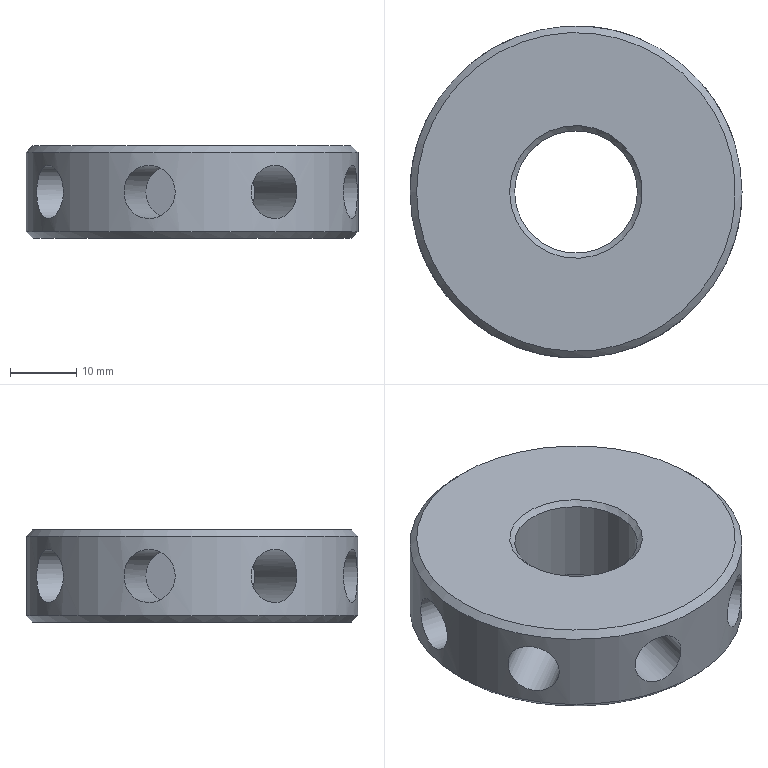Part | STEP file | 冲床-300配套压波_id1102_x_t | 1 solid | 24 faces | box 50 x 50 x 14 mm | volume 18346 mm3 | cylinder 10 | plane 10 | cone 4 | commonest cylinder face diameters 8 x8 18.5 x1 50 x1
STEP:
#1=CARTESIAN_POINT('',(1259.25,-86.,224.1));
#2=VERTEX_POINT('',#1);
#3=CARTESIAN_POINT('',(1250.,-86.,224.1));
#4=DIRECTION('',(0.,0.,-1.));
#5=DIRECTION('',(1.,0.,0.));
#6=AXIS2_PLACEMENT_3D('',#3,#4,#5);
#7=CIRCLE('',#6,9.25);
#8=EDGE_CURVE('',#2,#2,#7,.T.);
#9=ORIENTED_EDGE('',*,*,#8,.T.);
#10=EDGE_LOOP('',(#9));
#11=FACE_BOUND('',#10,.T.);
#12=CARTESIAN_POINT('',(1240.75,-86.,236.6));
#13=VERTEX_POINT('',#12);
#14=CARTESIAN_POINT('',(1250.,-86.,236.6));
#15=DIRECTION('',(0.,0.,1.));
#16=DIRECTION('',(-1.,0.,0.));
#17=AXIS2_PLACEMENT_3D('',#14,#15,#16);
#18=CIRCLE('',#17,9.25);
#19=EDGE_CURVE('',#13,#13,#18,.T.);
#20=ORIENTED_EDGE('',*,*,#19,.T.);
#21=EDGE_LOOP('',(#20));
#22=FACE_BOUND('',#21,.T.);
#23=CARTESIAN_POINT('',(1250.,-86.,224.35));
#24=DIRECTION('',(0.,0.,1.));
#25=DIRECTION('',(-1.,0.,0.));
#26=AXIS2_PLACEMENT_3D('',#23,#24,#25);
#27=CYLINDRICAL_SURFACE('',#26,9.25);
#28=ADVANCED_FACE('',(#11,#22),#27,.F.);
#29=CARTESIAN_POINT('',(1239.444,-79.03,230.35));
#30=VERTEX_POINT('',#29);
#31=CARTESIAN_POINT('',(1238.409,-82.894,230.35));
#32=DIRECTION('',(0.9659,-0.2588,0.));
#33=DIRECTION('',(0.2588,0.9659,0.));
#34=AXIS2_PLACEMENT_3D('',#31,#32,#33);
#35=CIRCLE('',#34,4.);
#36=EDGE_CURVE('',#30,#30,#35,.T.);
#37=ORIENTED_EDGE('',*,*,#36,.F.);
#38=EDGE_LOOP('',(#37));
#39=FACE_OUTER_BOUND('',#38,.T.);
#40=CARTESIAN_POINT('',(1238.409,-82.894,230.35));
#41=DIRECTION('',(0.9659,-0.2588,0.));
#42=DIRECTION('',(0.,0.,-1.));
#43=AXIS2_PLACEMENT_3D('',#40,#41,#42);
#44=PLANE('',#43);
#45=ADVANCED_FACE('',(#39),#44,.F.);
#46=CARTESIAN_POINT('',(1225.665,-80.271,234.276));
#47=VERTEX_POINT('',#46);
#48=CARTESIAN_POINT('',(1225.665,-80.271,234.276));
#49=CARTESIAN_POINT('',(1225.765,-79.848,234.361));
#50=CARTESIAN_POINT('',(1225.881,-79.407,234.372));
#51=CARTESIAN_POINT('',(1226.004,-78.986,234.31));
#52=CARTESIAN_POINT('',(1226.127,-78.566,234.248));
#53=CARTESIAN_POINT('',(1226.26,-78.153,234.11));
#54=CARTESIAN_POINT('',(1226.39,-77.781,233.908));
#55=CARTESIAN_POINT('',(1226.52,-77.407,233.705));
#56=CARTESIAN_POINT('',(1226.65,-77.064,233.432));
#57=CARTESIAN_POINT('',(1226.763,-76.777,233.111));
#58=CARTESIAN_POINT('',(1226.878,-76.488,232.786));
#59=CARTESIAN_POINT('',(1226.98,-76.248,232.404));
#60=CARTESIAN_POINT('',(1227.054,-76.077,231.995));
#61=CARTESIAN_POINT('',(1227.128,-75.906,231.586));
#62=CARTESIAN_POINT('',(1227.176,-75.798,231.139));
#63=CARTESIAN_POINT('',(1227.192,-75.763,230.691));
#64=CARTESIAN_POINT('',(1227.208,-75.728,230.249));
#65=CARTESIAN_POINT('',(1227.192,-75.762,229.793));
#66=CARTESIAN_POINT('',(1227.147,-75.864,229.363));
#67=CARTESIAN_POINT('',(1227.102,-75.964,228.935));
#68=CARTESIAN_POINT('',(1227.028,-76.134,228.52));
#69=CARTESIAN_POINT('',(1226.933,-76.36,228.151));
#70=CARTESIAN_POINT('',(1226.838,-76.588,227.779));
#71=CARTESIAN_POINT('',(1226.72,-76.879,227.444));
#72=CARTESIAN_POINT('',(1226.596,-77.212,227.174));
#73=CARTESIAN_POINT('',(1226.47,-77.547,226.901));
#74=CARTESIAN_POINT('',(1226.333,-77.934,226.686));
#75=CARTESIAN_POINT('',(1226.202,-78.342,226.546));
#76=CARTESIAN_POINT('',(1226.071,-78.747,226.408));
#77=CARTESIAN_POINT('',(1225.943,-79.185,226.341));
#78=CARTESIAN_POINT('',(1225.828,-79.618,226.351));
#79=CARTESIAN_POINT('',(1225.715,-80.046,226.361));
#80=CARTESIAN_POINT('',(1225.613,-80.481,226.447));
#81=CARTESIAN_POINT('',(1225.528,-80.888,226.601));
#82=CARTESIAN_POINT('',(1225.443,-81.295,226.756));
#83=CARTESIAN_POINT('',(1225.373,-81.683,226.983));
#84=CARTESIAN_POINT('',(1225.319,-82.022,227.264));
#85=CARTESIAN_POINT('',(1225.263,-82.364,227.549));
#86=CARTESIAN_POINT('',(1225.223,-82.664,227.896));
#87=CARTESIAN_POINT('',(1225.193,-82.896,228.278));
#88=CARTESIAN_POINT('',(1225.164,-83.129,228.663));
#89=CARTESIAN_POINT('',(1225.146,-83.299,229.093));
#90=CARTESIAN_POINT('',(1225.136,-83.392,229.534));
#91=CARTESIAN_POINT('',(1225.127,-83.483,229.97));
#92=CARTESIAN_POINT('',(1225.125,-83.501,230.429));
#93=CARTESIAN_POINT('',(1225.131,-83.442,230.871));
#94=CARTESIAN_POINT('',(1225.137,-83.384,231.31));
#95=CARTESIAN_POINT('',(1225.151,-83.25,231.744));
#96=CARTESIAN_POINT('',(1225.174,-83.052,232.139));
#97=CARTESIAN_POINT('',(1225.198,-82.853,232.535));
#98=CARTESIAN_POINT('',(1225.232,-82.584,232.903));
#99=CARTESIAN_POINT('',(1225.28,-82.268,233.213));
#100=CARTESIAN_POINT('',(1225.328,-81.949,233.526));
#101=CARTESIAN_POINT('',(1225.392,-81.574,233.788));
#102=CARTESIAN_POINT('',(1225.47,-81.173,233.977));
#103=CARTESIAN_POINT('',(1225.527,-80.885,234.113));
#104=CARTESIAN_POINT('',(1225.593,-80.58,234.214));
#105=CARTESIAN_POINT('',(1225.665,-80.271,234.276));
#106=B_SPLINE_CURVE_WITH_KNOTS('',3,(#48,#49,#50,#51,#52,#53,#54,#55,#56,#57,#58,#59,#60,#61,#62,#63,#64,#65,#66,#67,#68,#69,#70,#71,#72,#73,#74,#75,#76,#77,#78,#79,#80,#81,#82,#83,#84,#85,#86,#87,#88,#89,#90,#91,#92,#93,#94,#95,#96,#97,#98,#99,#100,#101,#102,#103,#104,#105),.UNSPECIFIED.,.T.,.F.,(1,3,3,3,3,3,3,3,3,3,3,3,3,3,3,3,3,3,3,3,3,1),(-0.03849,0.,0.05304,0.1061,0.1593,0.2132,0.267,0.3202,0.3732,0.4267,0.4806,0.5343,0.5873,0.6404,0.6941,0.748,0.8015,0.8544,0.9077,0.9615,1.,1.053),.UNSPECIFIED.);
#107=EDGE_CURVE('',#47,#47,#106,.T.);
#108=ORIENTED_EDGE('',*,*,#107,.T.);
#109=EDGE_LOOP('',(#108));
#110=FACE_BOUND('',#109,.T.);
#111=ORIENTED_EDGE('',*,*,#36,.T.);
#112=EDGE_LOOP('',(#111));
#113=FACE_BOUND('',#112,.T.);
#114=CARTESIAN_POINT('',(1233.579,-81.6,230.35));
#115=DIRECTION('',(0.9659,-0.2588,0.));
#116=DIRECTION('',(-0.2588,-0.9659,0.));
#117=AXIS2_PLACEMENT_3D('',#114,#115,#116);
#118=CYLINDRICAL_SURFACE('',#117,4.);
#119=ADVANCED_FACE('',(#110,#113),#118,.F.);
#120=CARTESIAN_POINT('',(1247.464,-73.608,230.35));
#121=VERTEX_POINT('',#120);
#122=CARTESIAN_POINT('',(1244.,-75.608,230.35));
#123=DIRECTION('',(0.5,-0.866,0.));
#124=DIRECTION('',(0.866,0.5,0.));
#125=AXIS2_PLACEMENT_3D('',#122,#123,#124);
#126=CIRCLE('',#125,4.);
#127=EDGE_CURVE('',#121,#121,#126,.T.);
#128=ORIENTED_EDGE('',*,*,#127,.F.);
#129=EDGE_LOOP('',(#128));
#130=FACE_OUTER_BOUND('',#129,.T.);
#131=CARTESIAN_POINT('',(1244.,-75.608,230.35));
#132=DIRECTION('',(0.5,-0.866,0.));
#133=DIRECTION('',(0.,0.,-1.));
#134=AXIS2_PLACEMENT_3D('',#131,#132,#133);
#135=PLANE('',#134);
#136=ADVANCED_FACE('',(#130),#135,.F.);
#137=CARTESIAN_POINT('',(1236.844,-64.742,234.276));
#138=VERTEX_POINT('',#137);
#139=CARTESIAN_POINT('',(1236.844,-64.742,234.276));
#140=CARTESIAN_POINT('',(1237.214,-64.513,234.361));
#141=CARTESIAN_POINT('',(1237.607,-64.284,234.372));
#142=CARTESIAN_POINT('',(1237.992,-64.073,234.31));
#143=CARTESIAN_POINT('',(1238.376,-63.862,234.248));
#144=CARTESIAN_POINT('',(1238.762,-63.665,234.11));
#145=CARTESIAN_POINT('',(1239.117,-63.493,233.908));
#146=CARTESIAN_POINT('',(1239.474,-63.321,233.705));
#147=CARTESIAN_POINT('',(1239.808,-63.17,233.432));
#148=CARTESIAN_POINT('',(1240.091,-63.048,233.111));
#149=CARTESIAN_POINT('',(1240.377,-62.924,232.786));
#150=CARTESIAN_POINT('',(1240.618,-62.827,232.404));
#151=CARTESIAN_POINT('',(1240.791,-62.758,231.995));
#152=CARTESIAN_POINT('',(1240.965,-62.689,231.586));
#153=CARTESIAN_POINT('',(1241.075,-62.647,231.139));
#154=CARTESIAN_POINT('',(1241.111,-62.634,230.691));
#155=CARTESIAN_POINT('',(1241.147,-62.62,230.249));
#156=CARTESIAN_POINT('',(1241.112,-62.633,229.793));
#157=CARTESIAN_POINT('',(1241.008,-62.673,229.363));
#158=CARTESIAN_POINT('',(1240.905,-62.713,228.935));
#159=CARTESIAN_POINT('',(1240.732,-62.78,228.52));
#160=CARTESIAN_POINT('',(1240.506,-62.873,228.151));
#161=CARTESIAN_POINT('',(1240.277,-62.967,227.779));
#162=CARTESIAN_POINT('',(1239.988,-63.089,227.444));
#163=CARTESIAN_POINT('',(1239.665,-63.236,227.174));
#164=CARTESIAN_POINT('',(1239.339,-63.384,226.901));
#165=CARTESIAN_POINT('',(1238.968,-63.561,226.686));
#166=CARTESIAN_POINT('',(1238.587,-63.757,226.546));
#167=CARTESIAN_POINT('',(1238.208,-63.951,226.408));
#168=CARTESIAN_POINT('',(1237.808,-64.17,226.341));
#169=CARTESIAN_POINT('',(1237.421,-64.395,226.351));
#170=CARTESIAN_POINT('',(1237.038,-64.618,226.361));
#171=CARTESIAN_POINT('',(1236.658,-64.854,226.447));
#172=CARTESIAN_POINT('',(1236.311,-65.081,226.601));
#173=CARTESIAN_POINT('',(1235.963,-65.309,226.756));
#174=CARTESIAN_POINT('',(1235.639,-65.534,226.983));
#175=CARTESIAN_POINT('',(1235.361,-65.734,227.264));
#176=CARTESIAN_POINT('',(1235.08,-65.937,227.549));
#177=CARTESIAN_POINT('',(1234.839,-66.121,227.896));
#178=CARTESIAN_POINT('',(1234.654,-66.264,228.278));
#179=CARTESIAN_POINT('',(1234.469,-66.408,228.663));
#180=CARTESIAN_POINT('',(1234.335,-66.516,229.093));
#181=CARTESIAN_POINT('',(1234.263,-66.575,229.534));
#182=CARTESIAN_POINT('',(1234.191,-66.633,229.97));
#183=CARTESIAN_POINT('',(1234.178,-66.644,230.429));
#184=CARTESIAN_POINT('',(1234.224,-66.606,230.871));
#185=CARTESIAN_POINT('',(1234.269,-66.57,231.31));
#186=CARTESIAN_POINT('',(1234.374,-66.485,231.744));
#187=CARTESIAN_POINT('',(1234.53,-66.361,232.139));
#188=CARTESIAN_POINT('',(1234.688,-66.237,232.535));
#189=CARTESIAN_POINT('',(1234.902,-66.071,232.903));
#190=CARTESIAN_POINT('',(1235.159,-65.882,233.213));
#191=CARTESIAN_POINT('',(1235.419,-65.69,233.526));
#192=CARTESIAN_POINT('',(1235.729,-65.469,233.788));
#193=CARTESIAN_POINT('',(1236.068,-65.242,233.977));
#194=CARTESIAN_POINT('',(1236.312,-65.078,234.113));
#195=CARTESIAN_POINT('',(1236.574,-64.909,234.214));
#196=CARTESIAN_POINT('',(1236.844,-64.742,234.276));
#197=B_SPLINE_CURVE_WITH_KNOTS('',3,(#139,#140,#141,#142,#143,#144,#145,#146,#147,#148,#149,#150,#151,#152,#153,#154,#155,#156,#157,#158,#159,#160,#161,#162,#163,#164,#165,#166,#167,#168,#169,#170,#171,#172,#173,#174,#175,#176,#177,#178,#179,#180,#181,#182,#183,#184,#185,#186,#187,#188,#189,#190,#191,#192,#193,#194,#195,#196),.UNSPECIFIED.,.T.,.F.,(1,3,3,3,3,3,3,3,3,3,3,3,3,3,3,3,3,3,3,3,3,1),(-0.03849,0.,0.05304,0.1061,0.1593,0.2132,0.267,0.3202,0.3732,0.4267,0.4806,0.5343,0.5873,0.6404,0.6941,0.748,0.8015,0.8544,0.9077,0.9615,1.,1.053),.UNSPECIFIED.);
#198=EDGE_CURVE('',#138,#138,#197,.T.);
#199=ORIENTED_EDGE('',*,*,#198,.T.);
#200=EDGE_LOOP('',(#199));
#201=FACE_BOUND('',#200,.T.);
#202=ORIENTED_EDGE('',*,*,#127,.T.);
#203=EDGE_LOOP('',(#202));
#204=FACE_BOUND('',#203,.T.);
#205=CARTESIAN_POINT('',(1241.5,-71.278,230.35));
#206=DIRECTION('',(0.5,-0.866,0.));
#207=DIRECTION('',(-0.866,-0.5,0.));
#208=AXIS2_PLACEMENT_3D('',#205,#206,#207);
#209=CYLINDRICAL_SURFACE('',#208,4.);
#210=ADVANCED_FACE('',(#201,#204),#209,.F.);
#211=CARTESIAN_POINT('',(1256.97,-75.444,230.35));
#212=VERTEX_POINT('',#211);
#213=CARTESIAN_POINT('',(1253.106,-74.409,230.35));
#214=DIRECTION('',(-0.2588,-0.9659,0.));
#215=DIRECTION('',(0.9659,-0.2588,0.));
#216=AXIS2_PLACEMENT_3D('',#213,#214,#215);
#217=CIRCLE('',#216,4.);
#218=EDGE_CURVE('',#212,#212,#217,.T.);
#219=ORIENTED_EDGE('',*,*,#218,.F.);
#220=EDGE_LOOP('',(#219));
#221=FACE_OUTER_BOUND('',#220,.T.);
#222=CARTESIAN_POINT('',(1253.106,-74.409,230.35));
#223=DIRECTION('',(-0.2588,-0.9659,0.));
#224=DIRECTION('',(0.,0.,-1.));
#225=AXIS2_PLACEMENT_3D('',#222,#223,#224);
#226=PLANE('',#225);
#227=ADVANCED_FACE('',(#221),#226,.F.);
#228=CARTESIAN_POINT('',(1255.729,-61.665,234.276));
#229=VERTEX_POINT('',#228);
#230=CARTESIAN_POINT('',(1255.729,-61.665,234.276));
#231=CARTESIAN_POINT('',(1256.152,-61.765,234.361));
#232=CARTESIAN_POINT('',(1256.593,-61.881,234.372));
#233=CARTESIAN_POINT('',(1257.014,-62.004,234.31));
#234=CARTESIAN_POINT('',(1257.434,-62.127,234.248));
#235=CARTESIAN_POINT('',(1257.847,-62.26,234.11));
#236=CARTESIAN_POINT('',(1258.219,-62.39,233.908));
#237=CARTESIAN_POINT('',(1258.593,-62.52,233.705));
#238=CARTESIAN_POINT('',(1258.936,-62.65,233.432));
#239=CARTESIAN_POINT('',(1259.223,-62.763,233.111));
#240=CARTESIAN_POINT('',(1259.512,-62.878,232.786));
#241=CARTESIAN_POINT('',(1259.752,-62.98,232.404));
#242=CARTESIAN_POINT('',(1259.923,-63.054,231.995));
#243=CARTESIAN_POINT('',(1260.094,-63.128,231.586));
#244=CARTESIAN_POINT('',(1260.202,-63.176,231.139));
#245=CARTESIAN_POINT('',(1260.237,-63.192,230.691));
#246=CARTESIAN_POINT('',(1260.272,-63.208,230.249));
#247=CARTESIAN_POINT('',(1260.238,-63.192,229.793));
#248=CARTESIAN_POINT('',(1260.136,-63.147,229.363));
#249=CARTESIAN_POINT('',(1260.036,-63.102,228.935));
#250=CARTESIAN_POINT('',(1259.866,-63.028,228.52));
#251=CARTESIAN_POINT('',(1259.64,-62.933,228.151));
#252=CARTESIAN_POINT('',(1259.412,-62.838,227.779));
#253=CARTESIAN_POINT('',(1259.121,-62.72,227.444));
#254=CARTESIAN_POINT('',(1258.788,-62.596,227.174));
#255=CARTESIAN_POINT('',(1258.453,-62.47,226.901));
#256=CARTESIAN_POINT('',(1258.066,-62.333,226.686));
#257=CARTESIAN_POINT('',(1257.658,-62.202,226.546));
#258=CARTESIAN_POINT('',(1257.253,-62.071,226.408));
#259=CARTESIAN_POINT('',(1256.815,-61.943,226.341));
#260=CARTESIAN_POINT('',(1256.382,-61.828,226.351));
#261=CARTESIAN_POINT('',(1255.954,-61.715,226.361));
#262=CARTESIAN_POINT('',(1255.519,-61.613,226.447));
#263=CARTESIAN_POINT('',(1255.112,-61.528,226.601));
#264=CARTESIAN_POINT('',(1254.705,-61.443,226.756));
#265=CARTESIAN_POINT('',(1254.317,-61.373,226.983));
#266=CARTESIAN_POINT('',(1253.978,-61.319,227.264));
#267=CARTESIAN_POINT('',(1253.636,-61.263,227.549));
#268=CARTESIAN_POINT('',(1253.336,-61.223,227.896));
#269=CARTESIAN_POINT('',(1253.104,-61.193,228.278));
#270=CARTESIAN_POINT('',(1252.871,-61.164,228.663));
#271=CARTESIAN_POINT('',(1252.701,-61.146,229.093));
#272=CARTESIAN_POINT('',(1252.608,-61.136,229.534));
#273=CARTESIAN_POINT('',(1252.517,-61.127,229.97));
#274=CARTESIAN_POINT('',(1252.499,-61.125,230.429));
#275=CARTESIAN_POINT('',(1252.558,-61.131,230.871));
#276=CARTESIAN_POINT('',(1252.616,-61.137,231.31));
#277=CARTESIAN_POINT('',(1252.75,-61.151,231.744));
#278=CARTESIAN_POINT('',(1252.948,-61.174,232.139));
#279=CARTESIAN_POINT('',(1253.147,-61.198,232.535));
#280=CARTESIAN_POINT('',(1253.416,-61.232,232.903));
#281=CARTESIAN_POINT('',(1253.732,-61.28,233.213));
#282=CARTESIAN_POINT('',(1254.051,-61.328,233.526));
#283=CARTESIAN_POINT('',(1254.426,-61.392,233.788));
#284=CARTESIAN_POINT('',(1254.827,-61.47,233.977));
#285=CARTESIAN_POINT('',(1255.115,-61.527,234.113));
#286=CARTESIAN_POINT('',(1255.42,-61.593,234.214));
#287=CARTESIAN_POINT('',(1255.729,-61.665,234.276));
#288=B_SPLINE_CURVE_WITH_KNOTS('',3,(#230,#231,#232,#233,#234,#235,#236,#237,#238,#239,#240,#241,#242,#243,#244,#245,#246,#247,#248,#249,#250,#251,#252,#253,#254,#255,#256,#257,#258,#259,#260,#261,#262,#263,#264,#265,#266,#267,#268,#269,#270,#271,#272,#273,#274,#275,#276,#277,#278,#279,#280,#281,#282,#283,#284,#285,#286,#287),.UNSPECIFIED.,.T.,.F.,(1,3,3,3,3,3,3,3,3,3,3,3,3,3,3,3,3,3,3,3,3,1),(-0.03849,0.,0.05304,0.1061,0.1593,0.2132,0.267,0.3202,0.3732,0.4267,0.4806,0.5343,0.5873,0.6404,0.6941,0.748,0.8015,0.8544,0.9077,0.9615,1.,1.053),.UNSPECIFIED.);
#289=EDGE_CURVE('',#229,#229,#288,.T.);
#290=ORIENTED_EDGE('',*,*,#289,.T.);
#291=EDGE_LOOP('',(#290));
#292=FACE_BOUND('',#291,.T.);
#293=ORIENTED_EDGE('',*,*,#218,.T.);
#294=EDGE_LOOP('',(#293));
#295=FACE_BOUND('',#294,.T.);
#296=CARTESIAN_POINT('',(1254.4,-69.579,230.35));
#297=DIRECTION('',(-0.2588,-0.9659,0.));
#298=DIRECTION('',(-0.9659,0.2588,0.));
#299=AXIS2_PLACEMENT_3D('',#296,#297,#298);
#300=CYLINDRICAL_SURFACE('',#299,4.);
#301=ADVANCED_FACE('',(#292,#295),#300,.F.);
#302=CARTESIAN_POINT('',(1262.392,-83.464,230.35));
#303=VERTEX_POINT('',#302);
#304=CARTESIAN_POINT('',(1260.392,-80.,230.35));
#305=DIRECTION('',(-0.866,-0.5,0.));
#306=DIRECTION('',(0.5,-0.866,0.));
#307=AXIS2_PLACEMENT_3D('',#304,#305,#306);
#308=CIRCLE('',#307,4.);
#309=EDGE_CURVE('',#303,#303,#308,.T.);
#310=ORIENTED_EDGE('',*,*,#309,.F.);
#311=EDGE_LOOP('',(#310));
#312=FACE_OUTER_BOUND('',#311,.T.);
#313=CARTESIAN_POINT('',(1260.392,-80.,230.35));
#314=DIRECTION('',(-0.866,-0.5,0.));
#315=DIRECTION('',(0.,0.,-1.));
#316=AXIS2_PLACEMENT_3D('',#313,#314,#315);
#317=PLANE('',#316);
#318=ADVANCED_FACE('',(#312),#317,.F.);
#319=CARTESIAN_POINT('',(1271.258,-72.844,234.276));
#320=VERTEX_POINT('',#319);
#321=CARTESIAN_POINT('',(1271.258,-72.844,234.276));
#322=CARTESIAN_POINT('',(1271.487,-73.214,234.361));
#323=CARTESIAN_POINT('',(1271.716,-73.607,234.372));
#324=CARTESIAN_POINT('',(1271.927,-73.992,234.31));
#325=CARTESIAN_POINT('',(1272.138,-74.376,234.248));
#326=CARTESIAN_POINT('',(1272.335,-74.762,234.11));
#327=CARTESIAN_POINT('',(1272.507,-75.117,233.908));
#328=CARTESIAN_POINT('',(1272.679,-75.474,233.705));
#329=CARTESIAN_POINT('',(1272.83,-75.808,233.432));
#330=CARTESIAN_POINT('',(1272.952,-76.091,233.111));
#331=CARTESIAN_POINT('',(1273.076,-76.377,232.786));
#332=CARTESIAN_POINT('',(1273.173,-76.618,232.404));
#333=CARTESIAN_POINT('',(1273.242,-76.791,231.995));
#334=CARTESIAN_POINT('',(1273.311,-76.965,231.586));
#335=CARTESIAN_POINT('',(1273.353,-77.075,231.139));
#336=CARTESIAN_POINT('',(1273.366,-77.111,230.691));
#337=CARTESIAN_POINT('',(1273.38,-77.147,230.249));
#338=CARTESIAN_POINT('',(1273.367,-77.112,229.793));
#339=CARTESIAN_POINT('',(1273.327,-77.008,229.363));
#340=CARTESIAN_POINT('',(1273.287,-76.905,228.935));
#341=CARTESIAN_POINT('',(1273.22,-76.732,228.52));
#342=CARTESIAN_POINT('',(1273.127,-76.506,228.151));
#343=CARTESIAN_POINT('',(1273.033,-76.277,227.779));
#344=CARTESIAN_POINT('',(1272.911,-75.988,227.444));
#345=CARTESIAN_POINT('',(1272.764,-75.665,227.174));
#346=CARTESIAN_POINT('',(1272.616,-75.339,226.901));
#347=CARTESIAN_POINT('',(1272.439,-74.968,226.686));
#348=CARTESIAN_POINT('',(1272.243,-74.587,226.546));
#349=CARTESIAN_POINT('',(1272.049,-74.208,226.408));
#350=CARTESIAN_POINT('',(1271.83,-73.808,226.341));
#351=CARTESIAN_POINT('',(1271.605,-73.421,226.351));
#352=CARTESIAN_POINT('',(1271.382,-73.038,226.361));
#353=CARTESIAN_POINT('',(1271.146,-72.658,226.447));
#354=CARTESIAN_POINT('',(1270.919,-72.311,226.601));
#355=CARTESIAN_POINT('',(1270.691,-71.963,226.756));
#356=CARTESIAN_POINT('',(1270.466,-71.639,226.983));
#357=CARTESIAN_POINT('',(1270.266,-71.361,227.264));
#358=CARTESIAN_POINT('',(1270.063,-71.08,227.549));
#359=CARTESIAN_POINT('',(1269.879,-70.839,227.896));
#360=CARTESIAN_POINT('',(1269.736,-70.654,228.278));
#361=CARTESIAN_POINT('',(1269.592,-70.469,228.663));
#362=CARTESIAN_POINT('',(1269.484,-70.335,229.093));
#363=CARTESIAN_POINT('',(1269.425,-70.263,229.534));
#364=CARTESIAN_POINT('',(1269.367,-70.191,229.97));
#365=CARTESIAN_POINT('',(1269.356,-70.178,230.429));
#366=CARTESIAN_POINT('',(1269.394,-70.224,230.871));
#367=CARTESIAN_POINT('',(1269.43,-70.269,231.31));
#368=CARTESIAN_POINT('',(1269.515,-70.374,231.744));
#369=CARTESIAN_POINT('',(1269.639,-70.53,232.139));
#370=CARTESIAN_POINT('',(1269.763,-70.688,232.535));
#371=CARTESIAN_POINT('',(1269.929,-70.902,232.903));
#372=CARTESIAN_POINT('',(1270.118,-71.159,233.213));
#373=CARTESIAN_POINT('',(1270.31,-71.419,233.526));
#374=CARTESIAN_POINT('',(1270.531,-71.729,233.788));
#375=CARTESIAN_POINT('',(1270.758,-72.068,233.977));
#376=CARTESIAN_POINT('',(1270.922,-72.312,234.113));
#377=CARTESIAN_POINT('',(1271.091,-72.574,234.214));
#378=CARTESIAN_POINT('',(1271.258,-72.844,234.276));
#379=B_SPLINE_CURVE_WITH_KNOTS('',3,(#321,#322,#323,#324,#325,#326,#327,#328,#329,#330,#331,#332,#333,#334,#335,#336,#337,#338,#339,#340,#341,#342,#343,#344,#345,#346,#347,#348,#349,#350,#351,#352,#353,#354,#355,#356,#357,#358,#359,#360,#361,#362,#363,#364,#365,#366,#367,#368,#369,#370,#371,#372,#373,#374,#375,#376,#377,#378),.UNSPECIFIED.,.T.,.F.,(1,3,3,3,3,3,3,3,3,3,3,3,3,3,3,3,3,3,3,3,3,1),(-0.03849,0.,0.05304,0.1061,0.1593,0.2132,0.267,0.3202,0.3732,0.4267,0.4806,0.5343,0.5873,0.6404,0.6941,0.748,0.8015,0.8544,0.9077,0.9615,1.,1.053),.UNSPECIFIED.);
#380=EDGE_CURVE('',#320,#320,#379,.T.);
#381=ORIENTED_EDGE('',*,*,#380,.T.);
#382=EDGE_LOOP('',(#381));
#383=FACE_BOUND('',#382,.T.);
#384=ORIENTED_EDGE('',*,*,#309,.T.);
#385=EDGE_LOOP('',(#384));
#386=FACE_BOUND('',#385,.T.);
#387=CARTESIAN_POINT('',(1264.722,-77.5,230.35));
#388=DIRECTION('',(-0.866,-0.5,0.));
#389=DIRECTION('',(-0.5,0.866,0.));
#390=AXIS2_PLACEMENT_3D('',#387,#388,#389);
#391=CYLINDRICAL_SURFACE('',#390,4.);
#392=ADVANCED_FACE('',(#383,#386),#391,.F.);
#393=CARTESIAN_POINT('',(1260.556,-92.97,230.35));
#394=VERTEX_POINT('',#393);
#395=CARTESIAN_POINT('',(1261.591,-89.106,230.35));
#396=DIRECTION('',(-0.9659,0.2588,0.));
#397=DIRECTION('',(-0.2588,-0.9659,0.));
#398=AXIS2_PLACEMENT_3D('',#395,#396,#397);
#399=CIRCLE('',#398,4.);
#400=EDGE_CURVE('',#394,#394,#399,.T.);
#401=ORIENTED_EDGE('',*,*,#400,.F.);
#402=EDGE_LOOP('',(#401));
#403=FACE_OUTER_BOUND('',#402,.T.);
#404=CARTESIAN_POINT('',(1261.591,-89.106,230.35));
#405=DIRECTION('',(-0.9659,0.2588,0.));
#406=DIRECTION('',(0.,0.,-1.));
#407=AXIS2_PLACEMENT_3D('',#404,#405,#406);
#408=PLANE('',#407);
#409=ADVANCED_FACE('',(#403),#408,.F.);
#410=CARTESIAN_POINT('',(1274.335,-91.729,234.276));
#411=VERTEX_POINT('',#410);
#412=CARTESIAN_POINT('',(1274.335,-91.729,234.276));
#413=CARTESIAN_POINT('',(1274.235,-92.152,234.361));
#414=CARTESIAN_POINT('',(1274.119,-92.593,234.372));
#415=CARTESIAN_POINT('',(1273.996,-93.014,234.31));
#416=CARTESIAN_POINT('',(1273.873,-93.434,234.248));
#417=CARTESIAN_POINT('',(1273.74,-93.847,234.11));
#418=CARTESIAN_POINT('',(1273.61,-94.219,233.908));
#419=CARTESIAN_POINT('',(1273.48,-94.593,233.705));
#420=CARTESIAN_POINT('',(1273.35,-94.936,233.432));
#421=CARTESIAN_POINT('',(1273.237,-95.223,233.111));
#422=CARTESIAN_POINT('',(1273.122,-95.512,232.786));
#423=CARTESIAN_POINT('',(1273.02,-95.752,232.404));
#424=CARTESIAN_POINT('',(1272.946,-95.923,231.995));
#425=CARTESIAN_POINT('',(1272.872,-96.094,231.586));
#426=CARTESIAN_POINT('',(1272.824,-96.202,231.139));
#427=CARTESIAN_POINT('',(1272.808,-96.237,230.691));
#428=CARTESIAN_POINT('',(1272.792,-96.272,230.249));
#429=CARTESIAN_POINT('',(1272.808,-96.238,229.793));
#430=CARTESIAN_POINT('',(1272.853,-96.136,229.363));
#431=CARTESIAN_POINT('',(1272.898,-96.036,228.935));
#432=CARTESIAN_POINT('',(1272.972,-95.866,228.52));
#433=CARTESIAN_POINT('',(1273.067,-95.64,228.151));
#434=CARTESIAN_POINT('',(1273.162,-95.412,227.779));
#435=CARTESIAN_POINT('',(1273.28,-95.121,227.444));
#436=CARTESIAN_POINT('',(1273.404,-94.788,227.174));
#437=CARTESIAN_POINT('',(1273.53,-94.453,226.901));
#438=CARTESIAN_POINT('',(1273.667,-94.066,226.686));
#439=CARTESIAN_POINT('',(1273.798,-93.658,226.546));
#440=CARTESIAN_POINT('',(1273.929,-93.253,226.408));
#441=CARTESIAN_POINT('',(1274.057,-92.815,226.341));
#442=CARTESIAN_POINT('',(1274.172,-92.382,226.351));
#443=CARTESIAN_POINT('',(1274.285,-91.954,226.361));
#444=CARTESIAN_POINT('',(1274.387,-91.519,226.447));
#445=CARTESIAN_POINT('',(1274.472,-91.112,226.601));
#446=CARTESIAN_POINT('',(1274.557,-90.705,226.756));
#447=CARTESIAN_POINT('',(1274.627,-90.317,226.983));
#448=CARTESIAN_POINT('',(1274.681,-89.978,227.264));
#449=CARTESIAN_POINT('',(1274.737,-89.636,227.549));
#450=CARTESIAN_POINT('',(1274.777,-89.336,227.896));
#451=CARTESIAN_POINT('',(1274.807,-89.104,228.278));
#452=CARTESIAN_POINT('',(1274.836,-88.871,228.663));
#453=CARTESIAN_POINT('',(1274.854,-88.701,229.093));
#454=CARTESIAN_POINT('',(1274.864,-88.608,229.534));
#455=CARTESIAN_POINT('',(1274.873,-88.517,229.97));
#456=CARTESIAN_POINT('',(1274.875,-88.499,230.429));
#457=CARTESIAN_POINT('',(1274.869,-88.558,230.871));
#458=CARTESIAN_POINT('',(1274.863,-88.616,231.31));
#459=CARTESIAN_POINT('',(1274.849,-88.75,231.744));
#460=CARTESIAN_POINT('',(1274.826,-88.948,232.139));
#461=CARTESIAN_POINT('',(1274.802,-89.147,232.535));
#462=CARTESIAN_POINT('',(1274.768,-89.416,232.903));
#463=CARTESIAN_POINT('',(1274.72,-89.732,233.213));
#464=CARTESIAN_POINT('',(1274.672,-90.051,233.526));
#465=CARTESIAN_POINT('',(1274.608,-90.426,233.788));
#466=CARTESIAN_POINT('',(1274.53,-90.827,233.977));
#467=CARTESIAN_POINT('',(1274.473,-91.115,234.113));
#468=CARTESIAN_POINT('',(1274.407,-91.42,234.214));
#469=CARTESIAN_POINT('',(1274.335,-91.729,234.276));
#470=B_SPLINE_CURVE_WITH_KNOTS('',3,(#412,#413,#414,#415,#416,#417,#418,#419,#420,#421,#422,#423,#424,#425,#426,#427,#428,#429,#430,#431,#432,#433,#434,#435,#436,#437,#438,#439,#440,#441,#442,#443,#444,#445,#446,#447,#448,#449,#450,#451,#452,#453,#454,#455,#456,#457,#458,#459,#460,#461,#462,#463,#464,#465,#466,#467,#468,#469),.UNSPECIFIED.,.T.,.F.,(1,3,3,3,3,3,3,3,3,3,3,3,3,3,3,3,3,3,3,3,3,1),(-0.03849,0.,0.05304,0.1061,0.1593,0.2132,0.267,0.3202,0.3732,0.4267,0.4806,0.5343,0.5873,0.6404,0.6941,0.748,0.8015,0.8544,0.9077,0.9615,1.,1.053),.UNSPECIFIED.);
#471=EDGE_CURVE('',#411,#411,#470,.T.);
#472=ORIENTED_EDGE('',*,*,#471,.T.);
#473=EDGE_LOOP('',(#472));
#474=FACE_BOUND('',#473,.T.);
#475=ORIENTED_EDGE('',*,*,#400,.T.);
#476=EDGE_LOOP('',(#475));
#477=FACE_BOUND('',#476,.T.);
#478=CARTESIAN_POINT('',(1266.421,-90.4,230.35));
#479=DIRECTION('',(-0.9659,0.2588,0.));
#480=DIRECTION('',(0.2588,0.9659,0.));
#481=AXIS2_PLACEMENT_3D('',#478,#479,#480);
#482=CYLINDRICAL_SURFACE('',#481,4.);
#483=ADVANCED_FACE('',(#474,#477),#482,.F.);
#484=CARTESIAN_POINT('',(1252.536,-98.392,230.35));
#485=VERTEX_POINT('',#484);
#486=CARTESIAN_POINT('',(1256.,-96.392,230.35));
#487=DIRECTION('',(-0.5,0.866,0.));
#488=DIRECTION('',(-0.866,-0.5,0.));
#489=AXIS2_PLACEMENT_3D('',#486,#487,#488);
#490=CIRCLE('',#489,4.);
#491=EDGE_CURVE('',#485,#485,#490,.T.);
#492=ORIENTED_EDGE('',*,*,#491,.F.);
#493=EDGE_LOOP('',(#492));
#494=FACE_OUTER_BOUND('',#493,.T.);
#495=CARTESIAN_POINT('',(1256.,-96.392,230.35));
#496=DIRECTION('',(-0.5,0.866,0.));
#497=DIRECTION('',(0.,0.,-1.));
#498=AXIS2_PLACEMENT_3D('',#495,#496,#497);
#499=PLANE('',#498);
#500=ADVANCED_FACE('',(#494),#499,.F.);
#501=CARTESIAN_POINT('',(1263.156,-107.258,234.276));
#502=VERTEX_POINT('',#501);
#503=CARTESIAN_POINT('',(1263.156,-107.258,234.276));
#504=CARTESIAN_POINT('',(1262.786,-107.487,234.361));
#505=CARTESIAN_POINT('',(1262.393,-107.716,234.372));
#506=CARTESIAN_POINT('',(1262.008,-107.927,234.31));
#507=CARTESIAN_POINT('',(1261.624,-108.138,234.248));
#508=CARTESIAN_POINT('',(1261.238,-108.335,234.11));
#509=CARTESIAN_POINT('',(1260.883,-108.507,233.908));
#510=CARTESIAN_POINT('',(1260.526,-108.679,233.705));
#511=CARTESIAN_POINT('',(1260.192,-108.83,233.432));
#512=CARTESIAN_POINT('',(1259.909,-108.952,233.111));
#513=CARTESIAN_POINT('',(1259.623,-109.076,232.786));
#514=CARTESIAN_POINT('',(1259.382,-109.173,232.404));
#515=CARTESIAN_POINT('',(1259.209,-109.242,231.995));
#516=CARTESIAN_POINT('',(1259.035,-109.311,231.586));
#517=CARTESIAN_POINT('',(1258.925,-109.353,231.139));
#518=CARTESIAN_POINT('',(1258.889,-109.366,230.691));
#519=CARTESIAN_POINT('',(1258.853,-109.38,230.249));
#520=CARTESIAN_POINT('',(1258.888,-109.367,229.793));
#521=CARTESIAN_POINT('',(1258.992,-109.327,229.363));
#522=CARTESIAN_POINT('',(1259.095,-109.287,228.935));
#523=CARTESIAN_POINT('',(1259.268,-109.22,228.52));
#524=CARTESIAN_POINT('',(1259.494,-109.127,228.151));
#525=CARTESIAN_POINT('',(1259.723,-109.033,227.779));
#526=CARTESIAN_POINT('',(1260.012,-108.911,227.444));
#527=CARTESIAN_POINT('',(1260.335,-108.764,227.174));
#528=CARTESIAN_POINT('',(1260.661,-108.616,226.901));
#529=CARTESIAN_POINT('',(1261.032,-108.439,226.686));
#530=CARTESIAN_POINT('',(1261.413,-108.243,226.546));
#531=CARTESIAN_POINT('',(1261.792,-108.049,226.408));
#532=CARTESIAN_POINT('',(1262.192,-107.83,226.341));
#533=CARTESIAN_POINT('',(1262.579,-107.605,226.351));
#534=CARTESIAN_POINT('',(1262.962,-107.382,226.361));
#535=CARTESIAN_POINT('',(1263.342,-107.146,226.447));
#536=CARTESIAN_POINT('',(1263.689,-106.919,226.601));
#537=CARTESIAN_POINT('',(1264.037,-106.691,226.756));
#538=CARTESIAN_POINT('',(1264.361,-106.466,226.983));
#539=CARTESIAN_POINT('',(1264.639,-106.266,227.264));
#540=CARTESIAN_POINT('',(1264.92,-106.063,227.549));
#541=CARTESIAN_POINT('',(1265.161,-105.879,227.896));
#542=CARTESIAN_POINT('',(1265.346,-105.736,228.278));
#543=CARTESIAN_POINT('',(1265.531,-105.592,228.663));
#544=CARTESIAN_POINT('',(1265.665,-105.484,229.093));
#545=CARTESIAN_POINT('',(1265.737,-105.425,229.534));
#546=CARTESIAN_POINT('',(1265.809,-105.367,229.97));
#547=CARTESIAN_POINT('',(1265.822,-105.356,230.429));
#548=CARTESIAN_POINT('',(1265.776,-105.394,230.871));
#549=CARTESIAN_POINT('',(1265.731,-105.43,231.31));
#550=CARTESIAN_POINT('',(1265.626,-105.515,231.744));
#551=CARTESIAN_POINT('',(1265.47,-105.639,232.139));
#552=CARTESIAN_POINT('',(1265.312,-105.763,232.535));
#553=CARTESIAN_POINT('',(1265.098,-105.929,232.903));
#554=CARTESIAN_POINT('',(1264.841,-106.118,233.213));
#555=CARTESIAN_POINT('',(1264.581,-106.31,233.526));
#556=CARTESIAN_POINT('',(1264.271,-106.531,233.788));
#557=CARTESIAN_POINT('',(1263.932,-106.758,233.977));
#558=CARTESIAN_POINT('',(1263.688,-106.922,234.113));
#559=CARTESIAN_POINT('',(1263.426,-107.091,234.214));
#560=CARTESIAN_POINT('',(1263.156,-107.258,234.276));
#561=B_SPLINE_CURVE_WITH_KNOTS('',3,(#503,#504,#505,#506,#507,#508,#509,#510,#511,#512,#513,#514,#515,#516,#517,#518,#519,#520,#521,#522,#523,#524,#525,#526,#527,#528,#529,#530,#531,#532,#533,#534,#535,#536,#537,#538,#539,#540,#541,#542,#543,#544,#545,#546,#547,#548,#549,#550,#551,#552,#553,#554,#555,#556,#557,#558,#559,#560),.UNSPECIFIED.,.T.,.F.,(1,3,3,3,3,3,3,3,3,3,3,3,3,3,3,3,3,3,3,3,3,1),(-0.03849,0.,0.05304,0.1061,0.1593,0.2132,0.267,0.3202,0.3732,0.4267,0.4806,0.5343,0.5873,0.6404,0.6941,0.748,0.8015,0.8544,0.9077,0.9615,1.,1.053),.UNSPECIFIED.);
#562=EDGE_CURVE('',#502,#502,#561,.T.);
#563=ORIENTED_EDGE('',*,*,#562,.T.);
#564=EDGE_LOOP('',(#563));
#565=FACE_BOUND('',#564,.T.);
#566=ORIENTED_EDGE('',*,*,#491,.T.);
#567=EDGE_LOOP('',(#566));
#568=FACE_BOUND('',#567,.T.);
#569=CARTESIAN_POINT('',(1258.5,-100.722,230.35));
#570=DIRECTION('',(-0.5,0.866,0.));
#571=DIRECTION('',(0.866,0.5,0.));
#572=AXIS2_PLACEMENT_3D('',#569,#570,#571);
#573=CYLINDRICAL_SURFACE('',#572,4.);
#574=ADVANCED_FACE('',(#565,#568),#573,.F.);
#575=CARTESIAN_POINT('',(1243.03,-96.556,230.35));
#576=VERTEX_POINT('',#575);
#577=CARTESIAN_POINT('',(1246.894,-97.591,230.35));
#578=DIRECTION('',(0.2588,0.9659,0.));
#579=DIRECTION('',(-0.9659,0.2588,0.));
#580=AXIS2_PLACEMENT_3D('',#577,#578,#579);
#581=CIRCLE('',#580,4.);
#582=EDGE_CURVE('',#576,#576,#581,.T.);
#583=ORIENTED_EDGE('',*,*,#582,.F.);
#584=EDGE_LOOP('',(#583));
#585=FACE_OUTER_BOUND('',#584,.T.);
#586=CARTESIAN_POINT('',(1246.894,-97.591,230.35));
#587=DIRECTION('',(0.2588,0.9659,0.));
#588=DIRECTION('',(0.,0.,-1.));
#589=AXIS2_PLACEMENT_3D('',#586,#587,#588);
#590=PLANE('',#589);
#591=ADVANCED_FACE('',(#585),#590,.F.);
#592=CARTESIAN_POINT('',(1244.271,-110.335,234.276));
#593=VERTEX_POINT('',#592);
#594=CARTESIAN_POINT('',(1244.271,-110.335,234.276));
#595=CARTESIAN_POINT('',(1243.848,-110.235,234.361));
#596=CARTESIAN_POINT('',(1243.407,-110.119,234.372));
#597=CARTESIAN_POINT('',(1242.986,-109.996,234.31));
#598=CARTESIAN_POINT('',(1242.566,-109.873,234.248));
#599=CARTESIAN_POINT('',(1242.153,-109.74,234.11));
#600=CARTESIAN_POINT('',(1241.781,-109.61,233.908));
#601=CARTESIAN_POINT('',(1241.407,-109.48,233.705));
#602=CARTESIAN_POINT('',(1241.064,-109.35,233.432));
#603=CARTESIAN_POINT('',(1240.777,-109.237,233.111));
#604=CARTESIAN_POINT('',(1240.488,-109.122,232.786));
#605=CARTESIAN_POINT('',(1240.248,-109.02,232.404));
#606=CARTESIAN_POINT('',(1240.077,-108.946,231.995));
#607=CARTESIAN_POINT('',(1239.906,-108.872,231.586));
#608=CARTESIAN_POINT('',(1239.798,-108.824,231.139));
#609=CARTESIAN_POINT('',(1239.763,-108.808,230.691));
#610=CARTESIAN_POINT('',(1239.728,-108.792,230.249));
#611=CARTESIAN_POINT('',(1239.762,-108.808,229.793));
#612=CARTESIAN_POINT('',(1239.864,-108.853,229.363));
#613=CARTESIAN_POINT('',(1239.964,-108.898,228.935));
#614=CARTESIAN_POINT('',(1240.134,-108.972,228.52));
#615=CARTESIAN_POINT('',(1240.36,-109.067,228.151));
#616=CARTESIAN_POINT('',(1240.588,-109.162,227.779));
#617=CARTESIAN_POINT('',(1240.879,-109.28,227.444));
#618=CARTESIAN_POINT('',(1241.212,-109.404,227.174));
#619=CARTESIAN_POINT('',(1241.547,-109.53,226.901));
#620=CARTESIAN_POINT('',(1241.934,-109.667,226.686));
#621=CARTESIAN_POINT('',(1242.342,-109.798,226.546));
#622=CARTESIAN_POINT('',(1242.747,-109.929,226.408));
#623=CARTESIAN_POINT('',(1243.185,-110.057,226.341));
#624=CARTESIAN_POINT('',(1243.618,-110.172,226.351));
#625=CARTESIAN_POINT('',(1244.046,-110.285,226.361));
#626=CARTESIAN_POINT('',(1244.481,-110.387,226.447));
#627=CARTESIAN_POINT('',(1244.888,-110.472,226.601));
#628=CARTESIAN_POINT('',(1245.295,-110.557,226.756));
#629=CARTESIAN_POINT('',(1245.683,-110.627,226.983));
#630=CARTESIAN_POINT('',(1246.022,-110.681,227.264));
#631=CARTESIAN_POINT('',(1246.364,-110.737,227.549));
#632=CARTESIAN_POINT('',(1246.664,-110.777,227.896));
#633=CARTESIAN_POINT('',(1246.896,-110.807,228.278));
#634=CARTESIAN_POINT('',(1247.129,-110.836,228.663));
#635=CARTESIAN_POINT('',(1247.299,-110.854,229.093));
#636=CARTESIAN_POINT('',(1247.392,-110.864,229.534));
#637=CARTESIAN_POINT('',(1247.483,-110.873,229.97));
#638=CARTESIAN_POINT('',(1247.501,-110.875,230.429));
#639=CARTESIAN_POINT('',(1247.442,-110.869,230.871));
#640=CARTESIAN_POINT('',(1247.384,-110.863,231.31));
#641=CARTESIAN_POINT('',(1247.25,-110.849,231.744));
#642=CARTESIAN_POINT('',(1247.052,-110.826,232.139));
#643=CARTESIAN_POINT('',(1246.853,-110.802,232.535));
#644=CARTESIAN_POINT('',(1246.584,-110.768,232.903));
#645=CARTESIAN_POINT('',(1246.268,-110.72,233.213));
#646=CARTESIAN_POINT('',(1245.949,-110.672,233.526));
#647=CARTESIAN_POINT('',(1245.574,-110.608,233.788));
#648=CARTESIAN_POINT('',(1245.173,-110.53,233.977));
#649=CARTESIAN_POINT('',(1244.885,-110.473,234.113));
#650=CARTESIAN_POINT('',(1244.58,-110.407,234.214));
#651=CARTESIAN_POINT('',(1244.271,-110.335,234.276));
#652=B_SPLINE_CURVE_WITH_KNOTS('',3,(#594,#595,#596,#597,#598,#599,#600,#601,#602,#603,#604,#605,#606,#607,#608,#609,#610,#611,#612,#613,#614,#615,#616,#617,#618,#619,#620,#621,#622,#623,#624,#625,#626,#627,#628,#629,#630,#631,#632,#633,#634,#635,#636,#637,#638,#639,#640,#641,#642,#643,#644,#645,#646,#647,#648,#649,#650,#651),.UNSPECIFIED.,.T.,.F.,(1,3,3,3,3,3,3,3,3,3,3,3,3,3,3,3,3,3,3,3,3,1),(-0.03849,0.,0.05304,0.1061,0.1593,0.2132,0.267,0.3202,0.3732,0.4267,0.4806,0.5343,0.5873,0.6404,0.6941,0.748,0.8015,0.8544,0.9077,0.9615,1.,1.053),.UNSPECIFIED.);
#653=EDGE_CURVE('',#593,#593,#652,.T.);
#654=ORIENTED_EDGE('',*,*,#653,.T.);
#655=EDGE_LOOP('',(#654));
#656=FACE_BOUND('',#655,.T.);
#657=ORIENTED_EDGE('',*,*,#582,.T.);
#658=EDGE_LOOP('',(#657));
#659=FACE_BOUND('',#658,.T.);
#660=CARTESIAN_POINT('',(1245.6,-102.421,230.35));
#661=DIRECTION('',(0.2588,0.9659,0.));
#662=DIRECTION('',(0.9659,-0.2588,0.));
#663=AXIS2_PLACEMENT_3D('',#660,#661,#662);
#664=CYLINDRICAL_SURFACE('',#663,4.);
#665=ADVANCED_FACE('',(#656,#659),#664,.F.);
#666=CARTESIAN_POINT('',(1240.,-86.,237.35));
#667=VERTEX_POINT('',#666);
#668=CARTESIAN_POINT('',(1250.,-86.,237.35));
#669=DIRECTION('',(0.,0.,-1.));
#670=DIRECTION('',(-1.,0.,0.));
#671=AXIS2_PLACEMENT_3D('',#668,#669,#670);
#672=CIRCLE('',#671,10.);
#673=EDGE_CURVE('',#667,#667,#672,.T.);
#674=ORIENTED_EDGE('',*,*,#673,.T.);
#675=EDGE_LOOP('',(#674));
#676=FACE_BOUND('',#675,.T.);
#677=CARTESIAN_POINT('',(1226.,-86.,237.35));
#678=VERTEX_POINT('',#677);
#679=CARTESIAN_POINT('',(1250.,-86.,237.35));
#680=DIRECTION('',(0.,0.,1.));
#681=DIRECTION('',(-1.,0.,0.));
#682=AXIS2_PLACEMENT_3D('',#679,#680,#681);
#683=CIRCLE('',#682,24.);
#684=EDGE_CURVE('',#678,#678,#683,.T.);
#685=ORIENTED_EDGE('',*,*,#684,.T.);
#686=EDGE_LOOP('',(#685));
#687=FACE_BOUND('',#686,.T.);
#688=CARTESIAN_POINT('',(1250.,-86.,237.35));
#689=DIRECTION('',(0.,0.,1.));
#690=DIRECTION('',(-1.,0.,0.));
#691=AXIS2_PLACEMENT_3D('',#688,#689,#690);
#692=PLANE('',#691);
#693=ADVANCED_FACE('',(#676,#687),#692,.T.);
#694=ORIENTED_EDGE('',*,*,#107,.F.);
#695=EDGE_LOOP('',(#694));
#696=FACE_BOUND('',#695,.T.);
#697=ORIENTED_EDGE('',*,*,#198,.F.);
#698=EDGE_LOOP('',(#697));
#699=FACE_BOUND('',#698,.T.);
#700=ORIENTED_EDGE('',*,*,#289,.F.);
#701=EDGE_LOOP('',(#700));
#702=FACE_BOUND('',#701,.T.);
#703=ORIENTED_EDGE('',*,*,#380,.F.);
#704=EDGE_LOOP('',(#703));
#705=FACE_BOUND('',#704,.T.);
#706=ORIENTED_EDGE('',*,*,#471,.F.);
#707=EDGE_LOOP('',(#706));
#708=FACE_BOUND('',#707,.T.);
#709=ORIENTED_EDGE('',*,*,#562,.F.);
#710=EDGE_LOOP('',(#709));
#711=FACE_BOUND('',#710,.T.);
#712=ORIENTED_EDGE('',*,*,#653,.F.);
#713=EDGE_LOOP('',(#712));
#714=FACE_BOUND('',#713,.T.);
#715=CARTESIAN_POINT('',(1225.,-86.,236.35));
#716=VERTEX_POINT('',#715);
#717=CARTESIAN_POINT('',(1250.,-86.,236.35));
#718=DIRECTION('',(0.,0.,-1.));
#719=DIRECTION('',(-1.,0.,0.));
#720=AXIS2_PLACEMENT_3D('',#717,#718,#719);
#721=CIRCLE('',#720,25.);
#722=EDGE_CURVE('',#716,#716,#721,.T.);
#723=ORIENTED_EDGE('',*,*,#722,.T.);
#724=EDGE_LOOP('',(#723));
#725=FACE_BOUND('',#724,.T.);
#726=CARTESIAN_POINT('',(1275.,-86.,224.35));
#727=VERTEX_POINT('',#726);
#728=CARTESIAN_POINT('',(1250.,-86.,224.35));
#729=DIRECTION('',(0.,0.,1.));
#730=DIRECTION('',(1.,0.,0.));
#731=AXIS2_PLACEMENT_3D('',#728,#729,#730);
#732=CIRCLE('',#731,25.);
#733=EDGE_CURVE('',#727,#727,#732,.T.);
#734=ORIENTED_EDGE('',*,*,#733,.T.);
#735=EDGE_LOOP('',(#734));
#736=FACE_BOUND('',#735,.T.);
#737=CARTESIAN_POINT('',(1228.742,-99.156,234.276));
#738=VERTEX_POINT('',#737);
#739=CARTESIAN_POINT('',(1228.742,-99.156,234.276));
#740=CARTESIAN_POINT('',(1228.513,-98.786,234.361));
#741=CARTESIAN_POINT('',(1228.284,-98.393,234.372));
#742=CARTESIAN_POINT('',(1228.073,-98.008,234.31));
#743=CARTESIAN_POINT('',(1227.862,-97.624,234.248));
#744=CARTESIAN_POINT('',(1227.665,-97.238,234.11));
#745=CARTESIAN_POINT('',(1227.493,-96.883,233.908));
#746=CARTESIAN_POINT('',(1227.321,-96.526,233.705));
#747=CARTESIAN_POINT('',(1227.17,-96.192,233.432));
#748=CARTESIAN_POINT('',(1227.048,-95.909,233.111));
#749=CARTESIAN_POINT('',(1226.924,-95.623,232.786));
#750=CARTESIAN_POINT('',(1226.827,-95.382,232.404));
#751=CARTESIAN_POINT('',(1226.758,-95.209,231.995));
#752=CARTESIAN_POINT('',(1226.689,-95.035,231.586));
#753=CARTESIAN_POINT('',(1226.647,-94.925,231.139));
#754=CARTESIAN_POINT('',(1226.634,-94.889,230.691));
#755=CARTESIAN_POINT('',(1226.62,-94.853,230.249));
#756=CARTESIAN_POINT('',(1226.633,-94.888,229.793));
#757=CARTESIAN_POINT('',(1226.673,-94.992,229.363));
#758=CARTESIAN_POINT('',(1226.713,-95.095,228.935));
#759=CARTESIAN_POINT('',(1226.78,-95.268,228.52));
#760=CARTESIAN_POINT('',(1226.873,-95.494,228.151));
#761=CARTESIAN_POINT('',(1226.967,-95.723,227.779));
#762=CARTESIAN_POINT('',(1227.089,-96.012,227.444));
#763=CARTESIAN_POINT('',(1227.236,-96.335,227.174));
#764=CARTESIAN_POINT('',(1227.384,-96.661,226.901));
#765=CARTESIAN_POINT('',(1227.561,-97.032,226.686));
#766=CARTESIAN_POINT('',(1227.757,-97.413,226.546));
#767=CARTESIAN_POINT('',(1227.951,-97.792,226.408));
#768=CARTESIAN_POINT('',(1228.17,-98.192,226.341));
#769=CARTESIAN_POINT('',(1228.395,-98.579,226.351));
#770=CARTESIAN_POINT('',(1228.618,-98.962,226.361));
#771=CARTESIAN_POINT('',(1228.854,-99.342,226.447));
#772=CARTESIAN_POINT('',(1229.081,-99.689,226.601));
#773=CARTESIAN_POINT('',(1229.309,-100.037,226.756));
#774=CARTESIAN_POINT('',(1229.534,-100.361,226.983));
#775=CARTESIAN_POINT('',(1229.734,-100.639,227.264));
#776=CARTESIAN_POINT('',(1229.937,-100.92,227.549));
#777=CARTESIAN_POINT('',(1230.121,-101.161,227.896));
#778=CARTESIAN_POINT('',(1230.264,-101.346,228.278));
#779=CARTESIAN_POINT('',(1230.408,-101.531,228.663));
#780=CARTESIAN_POINT('',(1230.516,-101.665,229.093));
#781=CARTESIAN_POINT('',(1230.575,-101.737,229.534));
#782=CARTESIAN_POINT('',(1230.633,-101.809,229.97));
#783=CARTESIAN_POINT('',(1230.644,-101.822,230.429));
#784=CARTESIAN_POINT('',(1230.606,-101.776,230.871));
#785=CARTESIAN_POINT('',(1230.57,-101.731,231.31));
#786=CARTESIAN_POINT('',(1230.485,-101.626,231.744));
#787=CARTESIAN_POINT('',(1230.361,-101.47,232.139));
#788=CARTESIAN_POINT('',(1230.237,-101.312,232.535));
#789=CARTESIAN_POINT('',(1230.071,-101.098,232.903));
#790=CARTESIAN_POINT('',(1229.882,-100.841,233.213));
#791=CARTESIAN_POINT('',(1229.69,-100.581,233.526));
#792=CARTESIAN_POINT('',(1229.469,-100.271,233.788));
#793=CARTESIAN_POINT('',(1229.242,-99.932,233.977));
#794=CARTESIAN_POINT('',(1229.078,-99.688,234.113));
#795=CARTESIAN_POINT('',(1228.909,-99.426,234.214));
#796=CARTESIAN_POINT('',(1228.742,-99.156,234.276));
#797=B_SPLINE_CURVE_WITH_KNOTS('',3,(#739,#740,#741,#742,#743,#744,#745,#746,#747,#748,#749,#750,#751,#752,#753,#754,#755,#756,#757,#758,#759,#760,#761,#762,#763,#764,#765,#766,#767,#768,#769,#770,#771,#772,#773,#774,#775,#776,#777,#778,#779,#780,#781,#782,#783,#784,#785,#786,#787,#788,#789,#790,#791,#792,#793,#794,#795,#796),.UNSPECIFIED.,.T.,.F.,(1,3,3,3,3,3,3,3,3,3,3,3,3,3,3,3,3,3,3,3,3,1),(-0.03849,0.,0.05304,0.1061,0.1593,0.2132,0.267,0.3202,0.3732,0.4267,0.4806,0.5343,0.5873,0.6404,0.6941,0.748,0.8015,0.8544,0.9077,0.9615,1.,1.053),.UNSPECIFIED.);
#798=EDGE_CURVE('',#738,#738,#797,.T.);
#799=ORIENTED_EDGE('',*,*,#798,.F.);
#800=EDGE_LOOP('',(#799));
#801=FACE_BOUND('',#800,.T.);
#802=CARTESIAN_POINT('',(1250.,-86.,234.35));
#803=DIRECTION('',(0.,0.,-1.));
#804=DIRECTION('',(1.,0.,0.));
#805=AXIS2_PLACEMENT_3D('',#802,#803,#804);
#806=CYLINDRICAL_SURFACE('',#805,25.);
#807=ADVANCED_FACE('',(#696,#699,#702,#705,#708,#711,#714,#725,#736,#801),#806,.T.);
#808=CARTESIAN_POINT('',(1260.,-86.,223.35));
#809=VERTEX_POINT('',#808);
#810=CARTESIAN_POINT('',(1250.,-86.,223.35));
#811=DIRECTION('',(0.,0.,1.));
#812=DIRECTION('',(1.,0.,0.));
#813=AXIS2_PLACEMENT_3D('',#810,#811,#812);
#814=CIRCLE('',#813,10.);
#815=EDGE_CURVE('',#809,#809,#814,.T.);
#816=ORIENTED_EDGE('',*,*,#815,.T.);
#817=EDGE_LOOP('',(#816));
#818=FACE_BOUND('',#817,.T.);
#819=CARTESIAN_POINT('',(1274.,-86.,223.35));
#820=VERTEX_POINT('',#819);
#821=CARTESIAN_POINT('',(1250.,-86.,223.35));
#822=DIRECTION('',(0.,0.,-1.));
#823=DIRECTION('',(1.,0.,0.));
#824=AXIS2_PLACEMENT_3D('',#821,#822,#823);
#825=CIRCLE('',#824,24.);
#826=EDGE_CURVE('',#820,#820,#825,.T.);
#827=ORIENTED_EDGE('',*,*,#826,.T.);
#828=EDGE_LOOP('',(#827));
#829=FACE_BOUND('',#828,.T.);
#830=CARTESIAN_POINT('',(1250.,-86.,223.35));
#831=DIRECTION('',(0.,0.,-1.));
#832=DIRECTION('',(1.,0.,0.));
#833=AXIS2_PLACEMENT_3D('',#830,#831,#832);
#834=PLANE('',#833);
#835=ADVANCED_FACE('',(#818,#829),#834,.T.);
#836=CARTESIAN_POINT('',(1237.608,-88.536,230.35));
#837=VERTEX_POINT('',#836);
#838=CARTESIAN_POINT('',(1239.608,-92.,230.35));
#839=DIRECTION('',(0.866,0.5,0.));
#840=DIRECTION('',(-0.5,0.866,0.));
#841=AXIS2_PLACEMENT_3D('',#838,#839,#840);
#842=CIRCLE('',#841,4.);
#843=EDGE_CURVE('',#837,#837,#842,.T.);
#844=ORIENTED_EDGE('',*,*,#843,.F.);
#845=EDGE_LOOP('',(#844));
#846=FACE_OUTER_BOUND('',#845,.T.);
#847=CARTESIAN_POINT('',(1239.608,-92.,230.35));
#848=DIRECTION('',(0.866,0.5,0.));
#849=DIRECTION('',(0.,0.,-1.));
#850=AXIS2_PLACEMENT_3D('',#847,#848,#849);
#851=PLANE('',#850);
#852=ADVANCED_FACE('',(#846),#851,.F.);
#853=ORIENTED_EDGE('',*,*,#798,.T.);
#854=EDGE_LOOP('',(#853));
#855=FACE_BOUND('',#854,.T.);
#856=ORIENTED_EDGE('',*,*,#843,.T.);
#857=EDGE_LOOP('',(#856));
#858=FACE_BOUND('',#857,.T.);
#859=CARTESIAN_POINT('',(1235.278,-94.5,230.35));
#860=DIRECTION('',(0.866,0.5,0.));
#861=DIRECTION('',(0.5,-0.866,0.));
#862=AXIS2_PLACEMENT_3D('',#859,#860,#861);
#863=CYLINDRICAL_SURFACE('',#862,4.);
#864=ADVANCED_FACE('',(#855,#858),#863,.F.);
#865=ORIENTED_EDGE('',*,*,#722,.F.);
#866=EDGE_LOOP('',(#865));
#867=FACE_BOUND('',#866,.T.);
#868=ORIENTED_EDGE('',*,*,#684,.F.);
#869=EDGE_LOOP('',(#868));
#870=FACE_BOUND('',#869,.T.);
#871=CARTESIAN_POINT('',(1250.,-86.,237.35));
#872=DIRECTION('',(0.,0.,-1.));
#873=DIRECTION('',(1.,0.,0.));
#874=AXIS2_PLACEMENT_3D('',#871,#872,#873);
#875=CONICAL_SURFACE('',#874,24.,45.);
#876=ADVANCED_FACE('',(#867,#870),#875,.T.);
#877=ORIENTED_EDGE('',*,*,#826,.F.);
#878=EDGE_LOOP('',(#877));
#879=FACE_BOUND('',#878,.T.);
#880=ORIENTED_EDGE('',*,*,#733,.F.);
#881=EDGE_LOOP('',(#880));
#882=FACE_BOUND('',#881,.T.);
#883=CARTESIAN_POINT('',(1250.,-86.,224.35));
#884=DIRECTION('',(0.,0.,1.));
#885=DIRECTION('',(-1.,0.,0.));
#886=AXIS2_PLACEMENT_3D('',#883,#884,#885);
#887=CONICAL_SURFACE('',#886,25.,45.);
#888=ADVANCED_FACE('',(#879,#882),#887,.T.);
#889=ORIENTED_EDGE('',*,*,#815,.F.);
#890=EDGE_LOOP('',(#889));
#891=FACE_BOUND('',#890,.T.);
#892=ORIENTED_EDGE('',*,*,#8,.F.);
#893=EDGE_LOOP('',(#892));
#894=FACE_BOUND('',#893,.T.);
#895=CARTESIAN_POINT('',(1250.,-86.,224.1));
#896=DIRECTION('',(0.,0.,-1.));
#897=DIRECTION('',(1.,0.,0.));
#898=AXIS2_PLACEMENT_3D('',#895,#896,#897);
#899=CONICAL_SURFACE('',#898,9.25,45.);
#900=ADVANCED_FACE('',(#891,#894),#899,.F.);
#901=ORIENTED_EDGE('',*,*,#673,.F.);
#902=EDGE_LOOP('',(#901));
#903=FACE_BOUND('',#902,.T.);
#904=ORIENTED_EDGE('',*,*,#19,.F.);
#905=EDGE_LOOP('',(#904));
#906=FACE_BOUND('',#905,.T.);
#907=CARTESIAN_POINT('',(1250.,-86.,236.6));
#908=DIRECTION('',(0.,0.,1.));
#909=DIRECTION('',(-1.,0.,0.));
#910=AXIS2_PLACEMENT_3D('',#907,#908,#909);
#911=CONICAL_SURFACE('',#910,9.25,45.);
#912=ADVANCED_FACE('',(#903,#906),#911,.F.);
#913=CLOSED_SHELL('',(#28,#45,#119,#136,#210,#227,#301,#318,#392,#409,#483,#500,#574,#591,#665,#693,#807,#835,#852,#864,#876,#888,#900,#912));
#914=MANIFOLD_SOLID_BREP('',#913);
#915=(LENGTH_UNIT()NAMED_UNIT(*)SI_UNIT(.MILLI.,.METRE.));
#916=UNCERTAINTY_MEASURE_WITH_UNIT(LENGTH_MEASURE(0.0508),#915,'','');
#917=(NAMED_UNIT(*)PLANE_ANGLE_UNIT()SI_UNIT($,.RADIAN.));
#918=PLANE_ANGLE_MEASURE_WITH_UNIT(PLANE_ANGLE_MEASURE(0.01745),#917);
#919=DIMENSIONAL_EXPONENTS(0.,0.,0.,0.,0.,0.,0.);
#920=(CONVERSION_BASED_UNIT('DEGREE',#918)NAMED_UNIT(#919)PLANE_ANGLE_UNIT());
#921=(NAMED_UNIT(*)SI_UNIT($,.STERADIAN.)SOLID_ANGLE_UNIT());
#922=(GEOMETRIC_REPRESENTATION_CONTEXT(3)GLOBAL_UNCERTAINTY_ASSIGNED_CONTEXT((#916))GLOBAL_UNIT_ASSIGNED_CONTEXT((#915,#920,#921))REPRESENTATION_CONTEXT('',''));
#923=ADVANCED_BREP_SHAPE_REPRESENTATION('',(#914),#922);